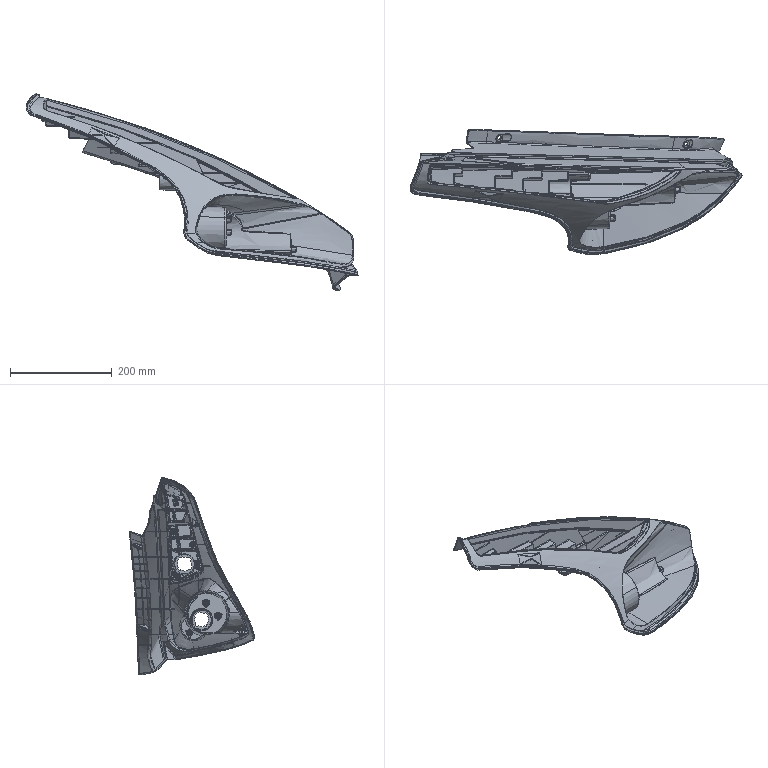Part | STEP file | solid 279 | 1 solid | 1877 faces | box 652.466 x 245.902 x 388.968 mm | volume 651328 mm3 | spline 1398 | plane 221 | sphere 87 | cylinder 75 | cone 45 | torus 44 | other 7 | commonest cylinder face diameters 2.01 x17 4.02 x17 27.135 x8 31.155 x8 2.915 x7 1.005 x6